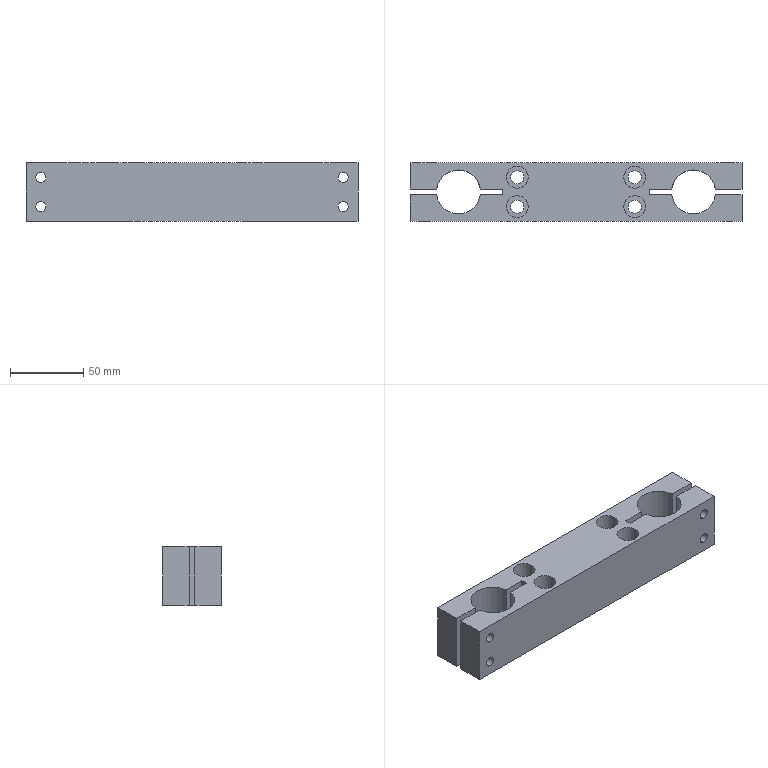Part | STEP file | 2002 Support shaft connecting plate | 1 solid | 70 faces | box 226 x 40 x 40 mm | volume 266231 mm3 | cylinder 44 | plane 26 | commonest cylinder face diameters 9 x16 15 x16 6.8 x8 30 x4